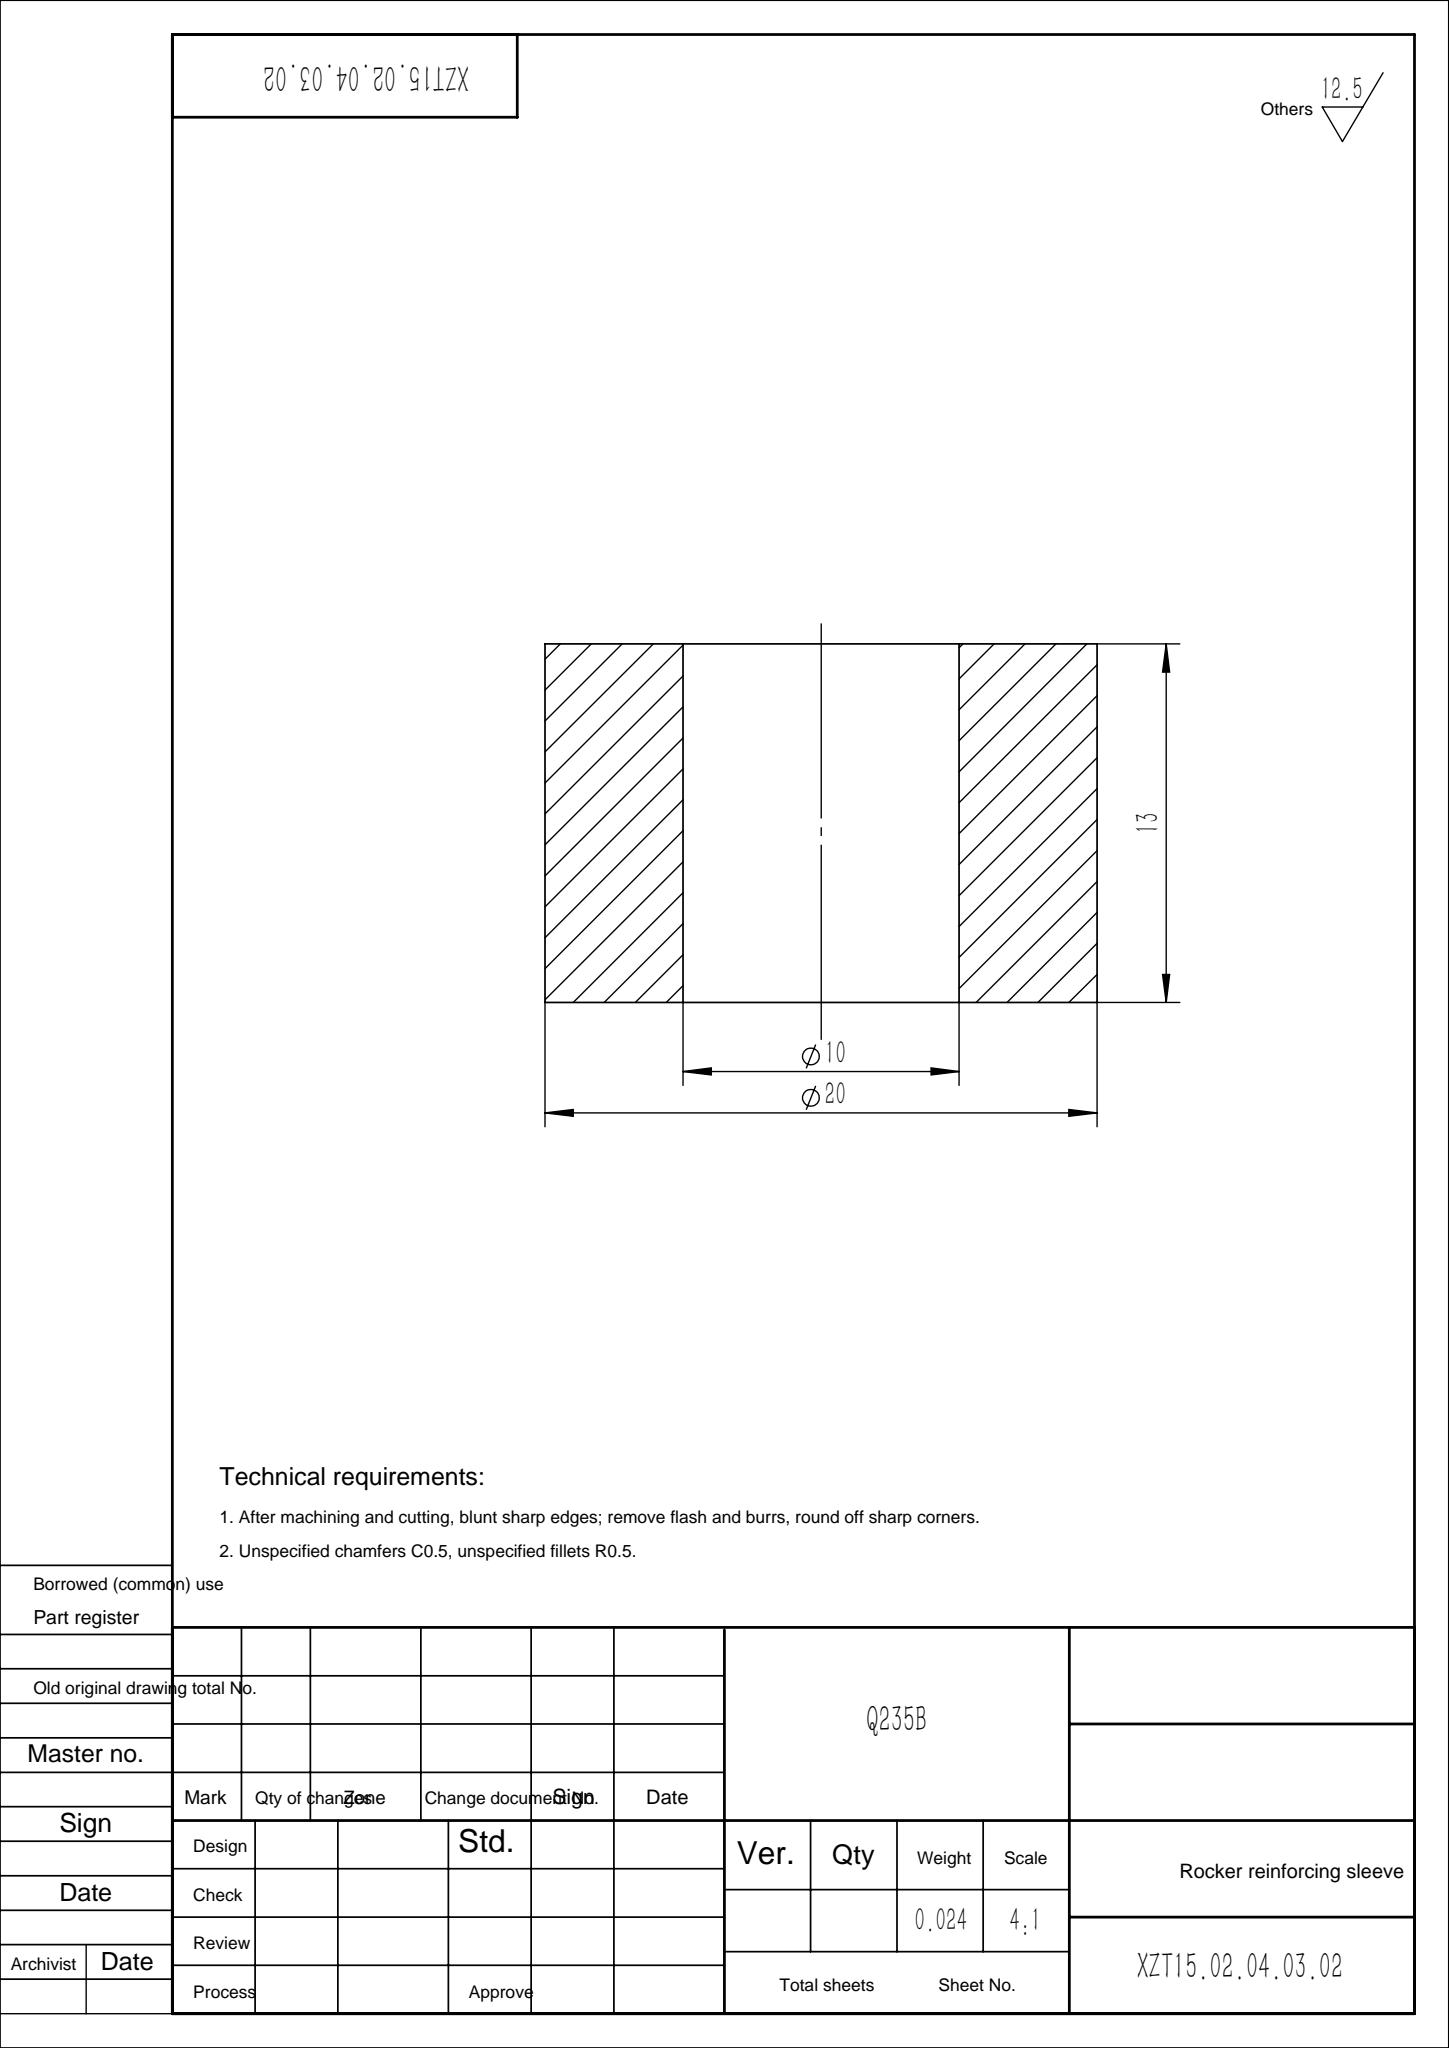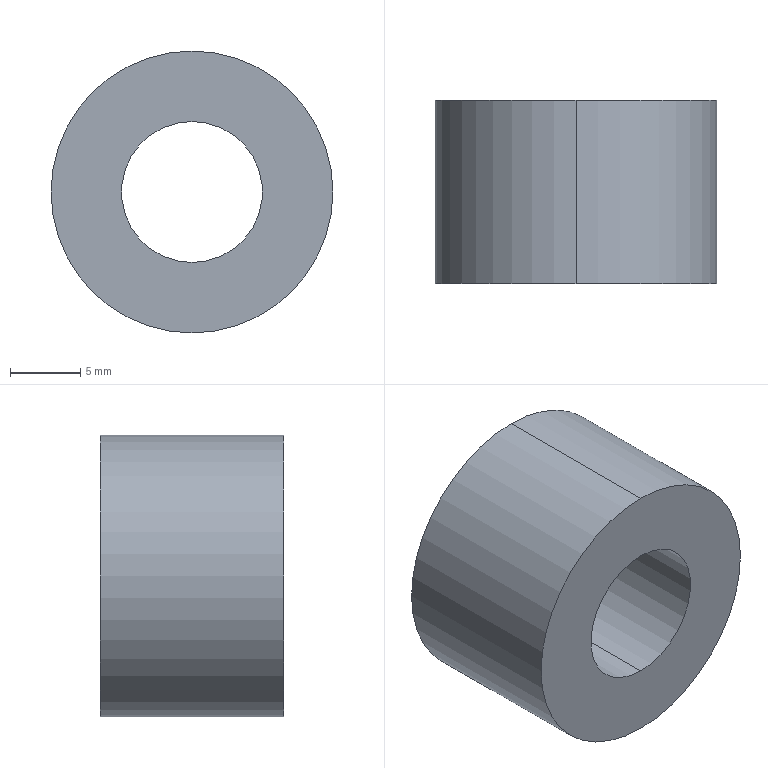Part | SolidWorks | features Extrusion 1 | 1 solid | 6 faces | box 20 x 13 x 20 mm | volume 3063 mm3 | cylinder 4 | plane 2 | commonest cylinder face diameters 10 x2 20 x2
STEP:
#1=CARTESIAN_POINT('',(0.,13.,-5.));
#2=VERTEX_POINT('',#1);
#3=CARTESIAN_POINT('',(0.,13.,5.));
#4=VERTEX_POINT('',#3);
#5=CARTESIAN_POINT('',(0.,13.,0.));
#6=DIRECTION('',(0.,1.,0.));
#7=DIRECTION('',(0.,0.,1.));
#8=AXIS2_PLACEMENT_3D('',#5,#6,#7);
#9=CIRCLE('',#8,5.);
#10=EDGE_CURVE('',#2,#4,#9,.T.);
#11=ORIENTED_EDGE('',*,*,#10,.T.);
#12=CARTESIAN_POINT('',(0.,0.,5.));
#13=VERTEX_POINT('',#12);
#14=CARTESIAN_POINT('',(0.,13.,5.));
#15=DIRECTION('',(0.,-1.,0.));
#16=VECTOR('',#15,1000.);
#17=LINE('',#14,#16);
#18=EDGE_CURVE('',#4,#13,#17,.T.);
#19=ORIENTED_EDGE('',*,*,#18,.T.);
#20=CARTESIAN_POINT('',(0.,0.,-5.));
#21=VERTEX_POINT('',#20);
#22=CARTESIAN_POINT('',(0.,0.,0.));
#23=DIRECTION('',(0.,1.,0.));
#24=DIRECTION('',(0.,0.,1.));
#25=AXIS2_PLACEMENT_3D('',#22,#23,#24);
#26=CIRCLE('',#25,5.);
#27=EDGE_CURVE('',#21,#13,#26,.T.);
#28=ORIENTED_EDGE('',*,*,#27,.F.);
#29=CARTESIAN_POINT('',(0.,13.,-5.));
#30=DIRECTION('',(0.,-1.,0.));
#31=VECTOR('',#30,1000.);
#32=LINE('',#29,#31);
#33=EDGE_CURVE('',#2,#21,#32,.T.);
#34=ORIENTED_EDGE('',*,*,#33,.F.);
#35=EDGE_LOOP('',(#11,#19,#28,#34));
#36=FACE_OUTER_BOUND('',#35,.T.);
#37=CARTESIAN_POINT('',(0.,13.,0.));
#38=DIRECTION('',(0.,-1.,0.));
#39=DIRECTION('',(0.,0.,-1.));
#40=AXIS2_PLACEMENT_3D('',#37,#38,#39);
#41=CYLINDRICAL_SURFACE('',#40,5.);
#42=ADVANCED_FACE('',(#36),#41,.F.);
#43=CARTESIAN_POINT('',(0.,13.,10.));
#44=VERTEX_POINT('',#43);
#45=CARTESIAN_POINT('',(0.,13.,-10.));
#46=VERTEX_POINT('',#45);
#47=CARTESIAN_POINT('',(0.,13.,0.));
#48=DIRECTION('',(0.,1.,0.));
#49=DIRECTION('',(0.,0.,1.));
#50=AXIS2_PLACEMENT_3D('',#47,#48,#49);
#51=CIRCLE('',#50,10.);
#52=EDGE_CURVE('',#44,#46,#51,.T.);
#53=ORIENTED_EDGE('',*,*,#52,.F.);
#54=CARTESIAN_POINT('',(0.,0.,10.));
#55=VERTEX_POINT('',#54);
#56=CARTESIAN_POINT('',(0.,13.,10.));
#57=DIRECTION('',(0.,-1.,0.));
#58=VECTOR('',#57,1000.);
#59=LINE('',#56,#58);
#60=EDGE_CURVE('',#44,#55,#59,.T.);
#61=ORIENTED_EDGE('',*,*,#60,.T.);
#62=CARTESIAN_POINT('',(0.,0.,-10.));
#63=VERTEX_POINT('',#62);
#64=CARTESIAN_POINT('',(0.,0.,0.));
#65=DIRECTION('',(0.,1.,0.));
#66=DIRECTION('',(0.,0.,1.));
#67=AXIS2_PLACEMENT_3D('',#64,#65,#66);
#68=CIRCLE('',#67,10.);
#69=EDGE_CURVE('',#55,#63,#68,.T.);
#70=ORIENTED_EDGE('',*,*,#69,.T.);
#71=CARTESIAN_POINT('',(0.,13.,-10.));
#72=DIRECTION('',(0.,-1.,0.));
#73=VECTOR('',#72,1000.);
#74=LINE('',#71,#73);
#75=EDGE_CURVE('',#46,#63,#74,.T.);
#76=ORIENTED_EDGE('',*,*,#75,.F.);
#77=EDGE_LOOP('',(#53,#61,#70,#76));
#78=FACE_OUTER_BOUND('',#77,.T.);
#79=CARTESIAN_POINT('',(0.,13.,0.));
#80=DIRECTION('',(0.,-1.,0.));
#81=DIRECTION('',(0.,0.,-1.));
#82=AXIS2_PLACEMENT_3D('',#79,#80,#81);
#83=CYLINDRICAL_SURFACE('',#82,10.);
#84=ADVANCED_FACE('',(#78),#83,.T.);
#85=CARTESIAN_POINT('',(0.,13.,0.));
#86=DIRECTION('',(0.,1.,0.));
#87=DIRECTION('',(0.,0.,1.));
#88=AXIS2_PLACEMENT_3D('',#85,#86,#87);
#89=CIRCLE('',#88,10.);
#90=EDGE_CURVE('',#46,#44,#89,.T.);
#91=ORIENTED_EDGE('',*,*,#90,.T.);
#92=ORIENTED_EDGE('',*,*,#52,.T.);
#93=EDGE_LOOP('',(#91,#92));
#94=FACE_OUTER_BOUND('',#93,.T.);
#95=ORIENTED_EDGE('',*,*,#10,.F.);
#96=CARTESIAN_POINT('',(0.,13.,0.));
#97=DIRECTION('',(0.,1.,0.));
#98=DIRECTION('',(0.,0.,1.));
#99=AXIS2_PLACEMENT_3D('',#96,#97,#98);
#100=CIRCLE('',#99,5.);
#101=EDGE_CURVE('',#4,#2,#100,.T.);
#102=ORIENTED_EDGE('',*,*,#101,.F.);
#103=EDGE_LOOP('',(#95,#102));
#104=FACE_BOUND('',#103,.T.);
#105=CARTESIAN_POINT('',(0.,13.,0.));
#106=DIRECTION('',(0.,1.,0.));
#107=DIRECTION('',(0.,0.,1.));
#108=AXIS2_PLACEMENT_3D('',#105,#106,#107);
#109=PLANE('',#108);
#110=ADVANCED_FACE('',(#94,#104),#109,.T.);
#111=CARTESIAN_POINT('',(0.,0.,0.));
#112=DIRECTION('',(0.,1.,0.));
#113=DIRECTION('',(0.,0.,1.));
#114=AXIS2_PLACEMENT_3D('',#111,#112,#113);
#115=CIRCLE('',#114,10.);
#116=EDGE_CURVE('',#63,#55,#115,.T.);
#117=ORIENTED_EDGE('',*,*,#116,.F.);
#118=ORIENTED_EDGE('',*,*,#69,.F.);
#119=EDGE_LOOP('',(#117,#118));
#120=FACE_OUTER_BOUND('',#119,.T.);
#121=ORIENTED_EDGE('',*,*,#27,.T.);
#122=CARTESIAN_POINT('',(0.,0.,0.));
#123=DIRECTION('',(0.,1.,0.));
#124=DIRECTION('',(0.,0.,1.));
#125=AXIS2_PLACEMENT_3D('',#122,#123,#124);
#126=CIRCLE('',#125,5.);
#127=EDGE_CURVE('',#13,#21,#126,.T.);
#128=ORIENTED_EDGE('',*,*,#127,.T.);
#129=EDGE_LOOP('',(#121,#128));
#130=FACE_BOUND('',#129,.T.);
#131=CARTESIAN_POINT('',(0.,0.,0.));
#132=DIRECTION('',(0.,1.,0.));
#133=DIRECTION('',(0.,0.,1.));
#134=AXIS2_PLACEMENT_3D('',#131,#132,#133);
#135=PLANE('',#134);
#136=ADVANCED_FACE('',(#120,#130),#135,.F.);
#137=ORIENTED_EDGE('',*,*,#60,.F.);
#138=ORIENTED_EDGE('',*,*,#90,.F.);
#139=ORIENTED_EDGE('',*,*,#75,.T.);
#140=ORIENTED_EDGE('',*,*,#116,.T.);
#141=EDGE_LOOP('',(#137,#138,#139,#140));
#142=FACE_OUTER_BOUND('',#141,.T.);
#143=CARTESIAN_POINT('',(0.,13.,0.));
#144=DIRECTION('',(0.,-1.,0.));
#145=DIRECTION('',(0.,0.,-1.));
#146=AXIS2_PLACEMENT_3D('',#143,#144,#145);
#147=CYLINDRICAL_SURFACE('',#146,10.);
#148=ADVANCED_FACE('',(#142),#147,.T.);
#149=ORIENTED_EDGE('',*,*,#18,.F.);
#150=ORIENTED_EDGE('',*,*,#101,.T.);
#151=ORIENTED_EDGE('',*,*,#33,.T.);
#152=ORIENTED_EDGE('',*,*,#127,.F.);
#153=EDGE_LOOP('',(#149,#150,#151,#152));
#154=FACE_OUTER_BOUND('',#153,.T.);
#155=CARTESIAN_POINT('',(0.,13.,0.));
#156=DIRECTION('',(0.,-1.,0.));
#157=DIRECTION('',(0.,0.,-1.));
#158=AXIS2_PLACEMENT_3D('',#155,#156,#157);
#159=CYLINDRICAL_SURFACE('',#158,5.);
#160=ADVANCED_FACE('',(#154),#159,.F.);
#161=CLOSED_SHELL('',(#42,#84,#110,#136,#148,#160));
#162=MANIFOLD_SOLID_BREP('',#161);
#163=CARTESIAN_POINT('',(0.,0.,0.));
#164=DIRECTION('',(0.,0.,1.));
#165=DIRECTION('',(1.,0.,0.));
#166=AXIS2_PLACEMENT_3D('',#163,#164,#165);
#167=(LENGTH_UNIT()NAMED_UNIT(*)SI_UNIT(.MILLI.,.METRE.));
#168=UNCERTAINTY_MEASURE_WITH_UNIT(LENGTH_MEASURE(0.00001),#167,'','');
#169=(NAMED_UNIT(*)PLANE_ANGLE_UNIT()SI_UNIT($,.RADIAN.));
#170=(NAMED_UNIT(*)SI_UNIT($,.STERADIAN.)SOLID_ANGLE_UNIT());
#171=(GEOMETRIC_REPRESENTATION_CONTEXT(3)GLOBAL_UNCERTAINTY_ASSIGNED_CONTEXT((#168))GLOBAL_UNIT_ASSIGNED_CONTEXT((#167,#169,#170))REPRESENTATION_CONTEXT('',''));
#172=ADVANCED_BREP_SHAPE_REPRESENTATION('',(#162,#166),#171);